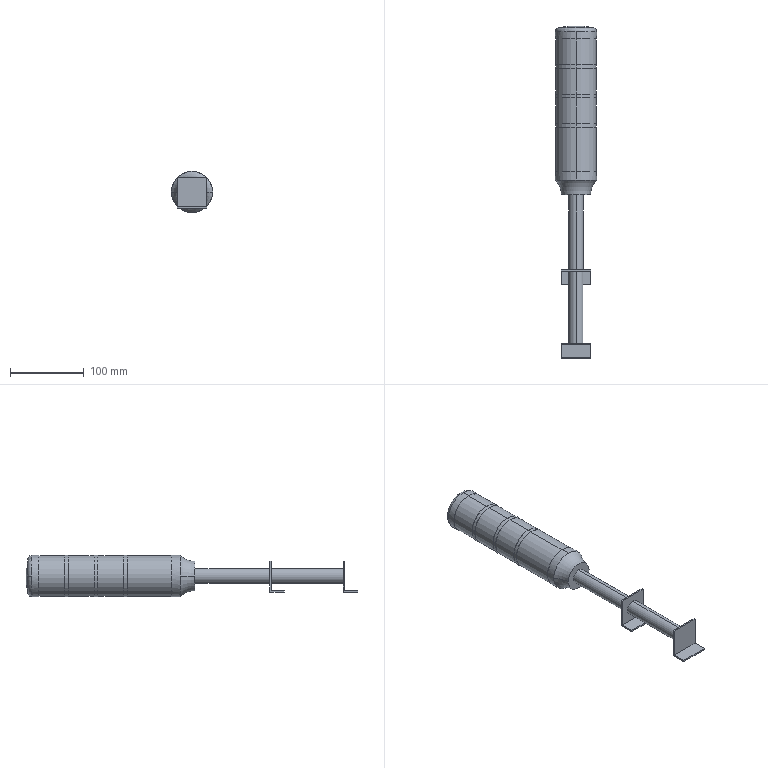Part | STEP file | Alarm light 3 | 1 solid | 52 faces | box 56 x 452 x 56 mm | volume 602047 mm3 | plane 25 | cylinder 22 | torus 4 | sphere 1 | commonest cylinder face diameters 56 x10 55 x8 20 x4